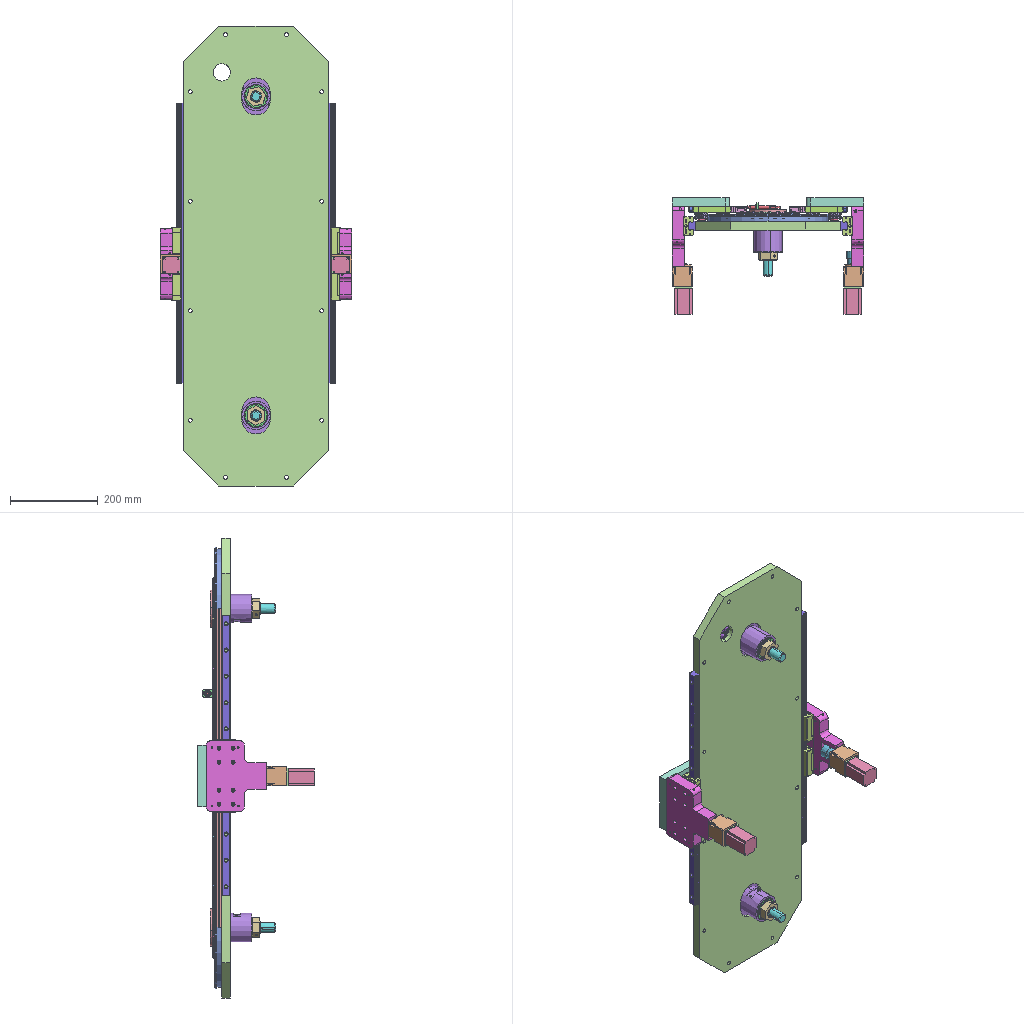Assembly | SolidWorks | 37 different items | 157 placed | box 436 x 267 x 1050 mm
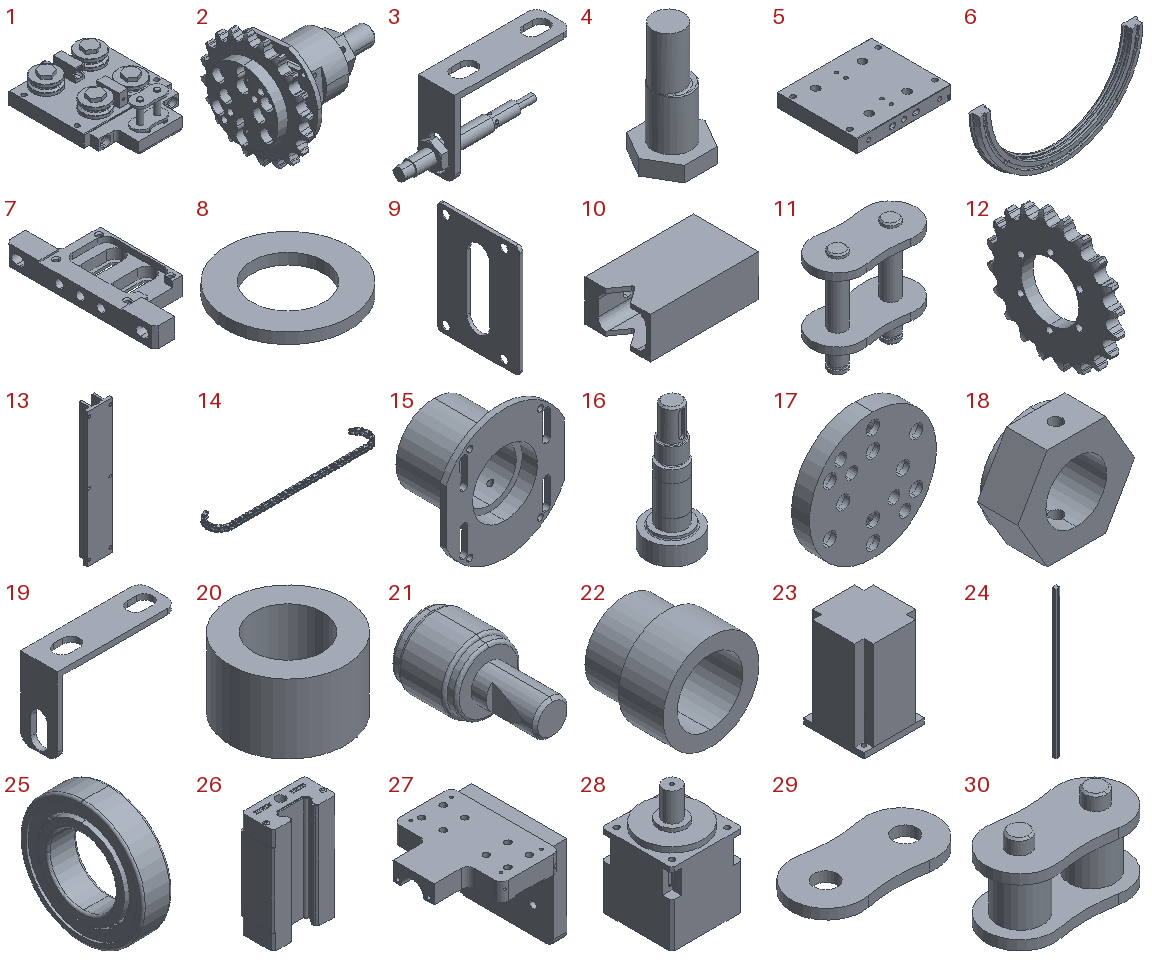Parts list (item | name | quantity | parent item | size | volume | features):
1 | (subassembly) | x2 | - | 100 x 133.3 x 40.5 mm | 173730 mm3 | features AEMSimFeature 1
2 | (subassembly) | x2 | - | 150 x 128.76 x 128.76 mm | 406242 mm3 | features AEMSimFeature 1
3 | (subassembly) | x1 | - | 86 x 20 x 43 mm | 8522 mm3 | features AEMSimFeature 1
4 | - | x4 | in 1 | 17.321 x 15 x 31.3 mm | 2525 mm3 | features BaseBody 1
5 | - | x2 | in 1 | 100 x 85 x 14 mm | 103040 mm3 | features BaseBody 1
6 | - | x2 | - | 280 x 16 x 140 mm | 112815 mm3 | features BaseBody 1
7 | - | x2 | in 1 | 37 x 90 x 12 mm | 17077 mm3 | features BaseBody 1
8 | - | x8 | in 1 | 18 x 18 x 1.6 mm | 268.606 mm3 | features BaseBody 1
9 | - | x2 | in 1 | 1.5 x 37 x 49.8 mm | 2125 mm3 | features BaseBody 1, ICE 1
10 | - | x4 | in 1 | 25 x 15.037 x 9.5 mm | 1907 mm3 | features BaseBody 1
11 | - | x2 | in 1 | 37.13 x 18.08 x 37.5 mm | 4809 mm3 | features BaseBody 1
12 | - | x2 | in 2 | 11.69 x 128.76 x 128.76 mm | 93096 mm3 | features BaseBody 1
13 | - | x2 | - | 49 x 25 x 260 mm | 106005 mm3 | features BaseBody 1
14 | - | x1 | - | 868.422 x 138.131 x 25.52 mm | 250514 mm3 | features BaseBody 84
15 | - | x2 | in 2 | 100 x 60 x 110 mm | 106856 mm3 | features BaseBody 1
16 | - | x2 | in 2 | 55 x 55 x 138 mm | 113601 mm3 | features BaseBody 1
17 | - | x2 | in 2 | 85 x 12 x 85 mm | 48417 mm3 | features BaseBody 1
18 | - | x2 | in 2 | 46.188 x 18 x 40 mm | 16224 mm3 | features BaseBody 1
19 | - | x1 | in 3 | 65 x 20 x 43 mm | 5123 mm3 | features BaseBody 1
20 | - | x4 | in 1 | 10 x 10 x 6 mm | 301.593 mm3 | features BaseBody 1
21 | - | x2 | in 1 | 12 x 22 x 12 mm | 1467 mm3 | features BaseBody 1
22 | - | x1 | - | 34.39 x 31 x 34.39 mm | 12104 mm3 | features BaseBody 1, Scale 1
23 | - | x2 | - | 40 x 40 x 78.25 mm | 93825 mm3 | features BaseBody 2, Scale 1
24 | - | x2 | - | 20 x 15.5 x 640 mm | 170066 mm3 | features BaseBody 1
25 | - | x4 | in 2 | 13 x 55 x 55 mm | 14062 mm3 | features BaseBody 1
26 | - | x4 | - | 42 x 22 x 70.1 mm | 49620 mm3 | features BaseBody 1
27 | - | x2 | - | 156.892 x 161 x 130 mm | 769090 mm3 | features ICE 9, Fillet 2, BaseBody 1, MoveFace 1
28 | - | x2 | - | 45 x 45 x 70.5 mm | 98334 mm3 | features BaseBody 1, Scale 1
29 | - | x38 | - | 37.13 x 18.08 x 2.59 mm | 1358 mm3 | features MoveFace 2, BaseBody 1
30 | - | x19 | - | 37.13 x 18.08 x 25.52 mm | 6230 mm3 | features MoveFace 2, BaseBody 1
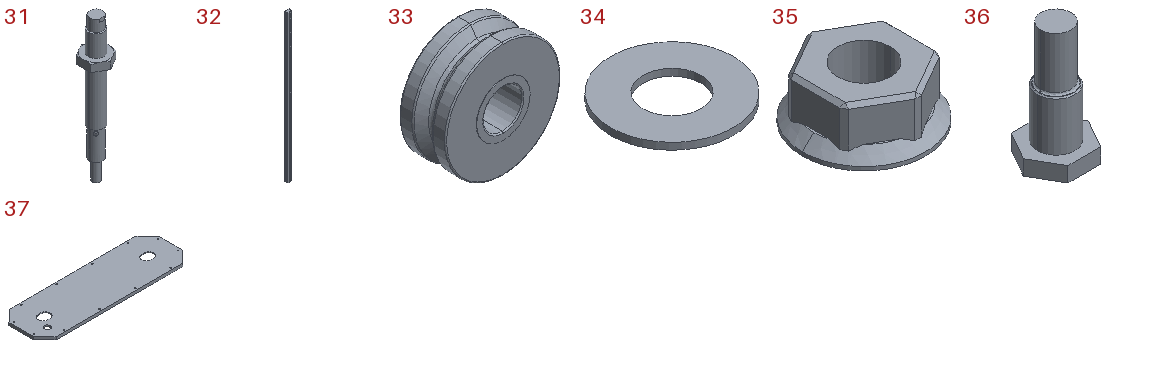31 | - | x1 | in 3 | 13 x 15.011 x 74 mm | 3399 mm3 | features BaseBody 2
32 | - | x2 | - | 25 x 16 x 728 mm | 224538 mm3 | features BaseBody 1
33 | - | x8 | in 1 | 29.5 x 12 x 29.5 mm | 6423 mm3 | features BaseBody 1
34 | - | x8 | in 1 | 18 x 18 x 1 mm | 197.724 mm3 | features BaseBody 1
35 | - | x8 | in 1 | 16.4 x 16.4 x 6.8 mm | 790.992 mm3 | features BaseBody 1
36 | - | x4 | in 1 | 17.321 x 15 x 31.3 mm | 2525 mm3 | features BaseBody 1
37 | - | x1 | - | 1050 x 330 x 20 mm | 5286047 mm3 | features BaseBody 1
Mates (type | each side: item.copy, entity, surface, feature):
Slot | 37.1 face cylinder Import1 | 15.1 face cylinder Import1
Coincident | 37.1 face plane Import1 | 15.1 face plane Import1
Slot | 37.1 face plane Import1 | 15.2 face cylinder Import1
Coincident | 37.1 face plane Import1 | 15.2 face plane Import1
Coincident | 27.1 face plane Import1 | 28.1 face plane Import1 | 2 times
Concentric | 28.1 face cylinder Import1 | 22.1 face cylinder Import1
Coincident | 28.1 face plane Import1 | 22.1 face plane Import1
Coincident | 28.1 face plane Import1 | 23.1 face plane Import2
DistanceDim | 23.1 face plane Import2 | 28.1 face plane Import1
DistanceDim | 28.1 face plane Import1 | 23.1 face plane Import2
Coincident | 37.1 face plane Import1 | 24.1 face plane Import1
Parallel | 37.1 face plane Import1 | 24.1 face plane Import1
Parallel | 27.1 face cylinder Cut-Extrude 3 | 22.1 face cylinder Import1
DistanceDim | 27.1 face plane Cut-Extrude 2 | 28.1 face plane Import1
Coincident | 27.1 face plane Import1 | 26.1 face plane Import1
Coincident | 26.2 face plane Import1 | 27.1 face plane Import1
Concentric | 27.1 face cylinder Import1 | 26.1 face cylinder Import1 | 2 times
Concentric | 26.2 face cylinder Import1 | 27.1 face cylinder Import1 | 2 times
Coincident | 24.1 face plane Import1 | 26.1 face plane Import1 | 2 times
Coincident | 5.1 face plane Import1 | 27.1 face plane Boss-Extrude 3
Concentric | 5.1 face cylinder Import1 | 27.1 face cylinder Cut-Extrude 6 | 2 times
Coincident | 5.2 face plane Import1 | 27.2 face plane Boss-Extrude 3
Concentric | 5.2 face cylinder Import1 | 27.2 face cylinder Cut-Extrude 6 | 2 times